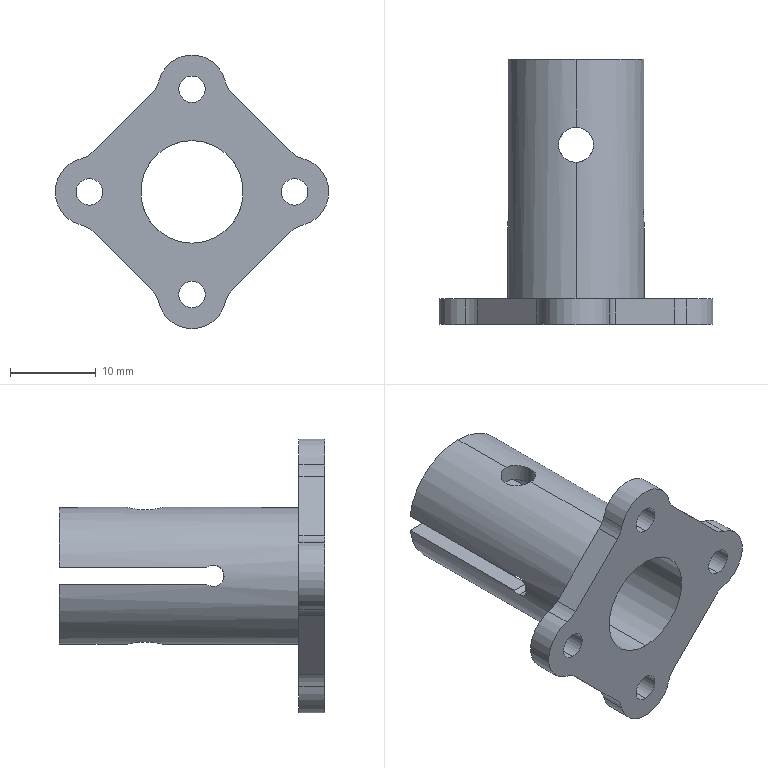Part | SolidWorks | features ICE 3, Extrusion 1, Fillet 1 | 1 solid | 47 faces | box 32 x 31 x 32 mm | volume 3496 mm3 | cylinder 35 | plane 12 | commonest cylinder face diameters 3.1 x8 6 x8 2.5 x6 8 x5 4.1 x4 12 x2